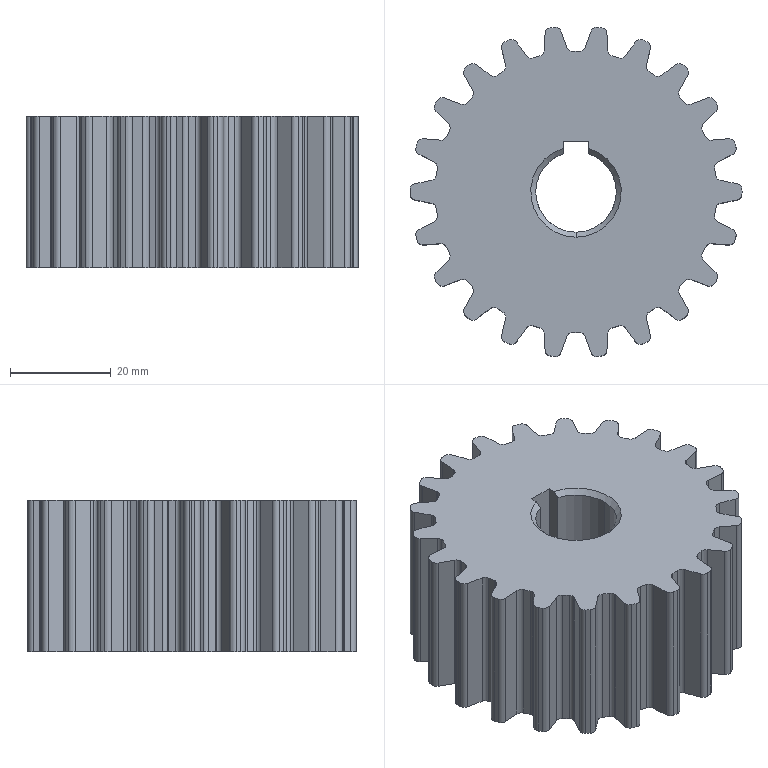Part | STEP file | Driving pulley | 1 solid | 206 faces | box 65.94 x 65.413 x 30 mm | volume 79962 mm3 | cylinder 130 | plane 71 | cone 5 | commonest cylinder face diameters 2.34 x52 2.38 x52 65.94 x23 16 x3